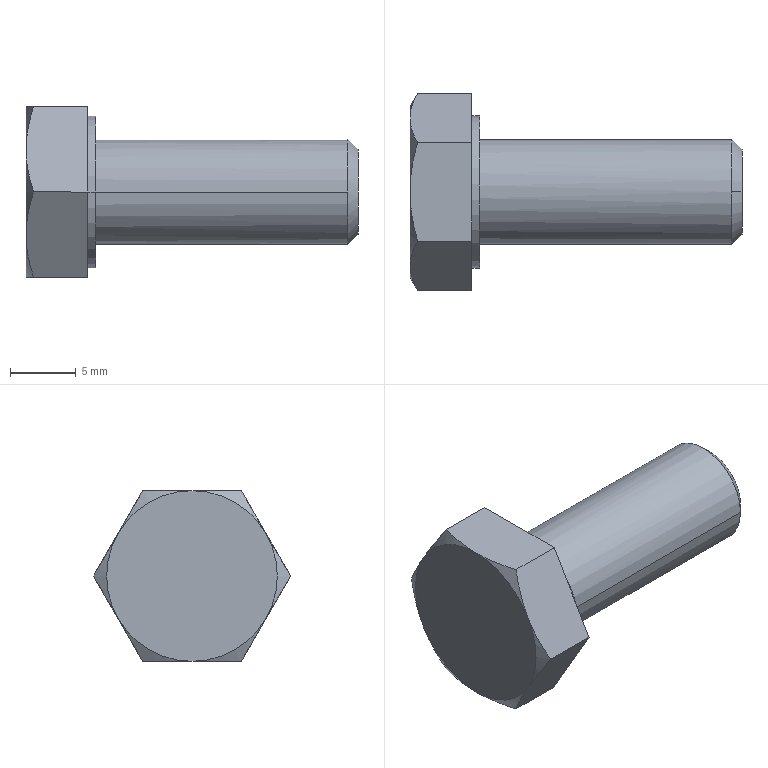Part | SolidWorks | features BaseBody 1 | 1 solid | 22 faces | box 25.3 x 15.011 x 13 mm | volume 1747 mm3 | plane 10 | cone 8 | cylinder 4 | commonest cylinder face diameters 8 x2 11.6 x2
STEP:
#1=CARTESIAN_POINT('',(0.,4.,0.));
#2=VERTEX_POINT('',#1);
#3=CARTESIAN_POINT('',(0.,-4.,0.));
#4=VERTEX_POINT('',#3);
#5=CARTESIAN_POINT('',(0.,0.,0.));
#6=DIRECTION('',(1.,0.,0.));
#7=DIRECTION('',(0.,1.,0.));
#8=AXIS2_PLACEMENT_3D('',#5,#6,#7);
#9=CIRCLE('',#8,4.);
#10=EDGE_CURVE('',#2,#4,#9,.T.);
#11=ORIENTED_EDGE('',*,*,#10,.T.);
#12=CARTESIAN_POINT('',(19.233,-4.,0.));
#13=VERTEX_POINT('',#12);
#14=CARTESIAN_POINT('',(10.625,-4.,0.));
#15=DIRECTION('',(1.,0.,0.));
#16=VECTOR('',#15,1000.);
#17=LINE('',#14,#16);
#18=EDGE_CURVE('',#4,#13,#17,.T.);
#19=ORIENTED_EDGE('',*,*,#18,.T.);
#20=CARTESIAN_POINT('',(19.233,0.,4.));
#21=VERTEX_POINT('',#20);
#22=CARTESIAN_POINT('',(19.233,0.,0.));
#23=DIRECTION('',(-1.,0.,0.));
#24=DIRECTION('',(0.,1.,0.));
#25=AXIS2_PLACEMENT_3D('',#22,#23,#24);
#26=CIRCLE('',#25,4.);
#27=EDGE_CURVE('',#13,#21,#26,.T.);
#28=ORIENTED_EDGE('',*,*,#27,.T.);
#29=CARTESIAN_POINT('',(19.233,4.,0.));
#30=VERTEX_POINT('',#29);
#31=CARTESIAN_POINT('',(19.233,0.,0.));
#32=DIRECTION('',(-1.,0.,0.));
#33=DIRECTION('',(0.,1.,0.));
#34=AXIS2_PLACEMENT_3D('',#31,#32,#33);
#35=CIRCLE('',#34,4.);
#36=EDGE_CURVE('',#21,#30,#35,.T.);
#37=ORIENTED_EDGE('',*,*,#36,.T.);
#38=CARTESIAN_POINT('',(10.625,4.,0.));
#39=DIRECTION('',(1.,0.,0.));
#40=VECTOR('',#39,1000.);
#41=LINE('',#38,#40);
#42=EDGE_CURVE('',#2,#30,#41,.T.);
#43=ORIENTED_EDGE('',*,*,#42,.F.);
#44=EDGE_LOOP('',(#11,#19,#28,#37,#43));
#45=FACE_OUTER_BOUND('',#44,.T.);
#46=CARTESIAN_POINT('',(10.625,0.,0.));
#47=DIRECTION('',(1.,0.,0.));
#48=DIRECTION('',(0.,1.,0.));
#49=AXIS2_PLACEMENT_3D('',#46,#47,#48);
#50=CYLINDRICAL_SURFACE('',#49,4.);
#51=ADVANCED_FACE('',(#45),#50,.T.);
#52=CARTESIAN_POINT('',(20.,0.,3.233));
#53=VERTEX_POINT('',#52);
#54=CARTESIAN_POINT('',(20.,0.,-3.233));
#55=VERTEX_POINT('',#54);
#56=CARTESIAN_POINT('',(20.,0.,0.));
#57=DIRECTION('',(-1.,0.,0.));
#58=DIRECTION('',(0.,0.,1.));
#59=AXIS2_PLACEMENT_3D('',#56,#57,#58);
#60=CIRCLE('',#59,3.233);
#61=EDGE_CURVE('',#53,#55,#60,.T.);
#62=ORIENTED_EDGE('',*,*,#61,.T.);
#63=CARTESIAN_POINT('',(19.233,0.,-4.));
#64=VERTEX_POINT('',#63);
#65=CARTESIAN_POINT('',(19.233,0.,-4.));
#66=DIRECTION('',(-0.7072,0.,-0.7071));
#67=VECTOR('',#66,1000.);
#68=LINE('',#65,#67);
#69=EDGE_CURVE('',#55,#64,#68,.T.);
#70=ORIENTED_EDGE('',*,*,#69,.T.);
#71=CARTESIAN_POINT('',(19.233,0.,0.));
#72=DIRECTION('',(-1.,0.,0.));
#73=DIRECTION('',(0.,1.,0.));
#74=AXIS2_PLACEMENT_3D('',#71,#72,#73);
#75=CIRCLE('',#74,4.);
#76=EDGE_CURVE('',#30,#64,#75,.T.);
#77=ORIENTED_EDGE('',*,*,#76,.F.);
#78=ORIENTED_EDGE('',*,*,#36,.F.);
#79=CARTESIAN_POINT('',(19.233,0.,4.));
#80=DIRECTION('',(-0.7072,0.,0.7071));
#81=VECTOR('',#80,1000.);
#82=LINE('',#79,#81);
#83=EDGE_CURVE('',#53,#21,#82,.T.);
#84=ORIENTED_EDGE('',*,*,#83,.F.);
#85=EDGE_LOOP('',(#62,#70,#77,#78,#84));
#86=FACE_OUTER_BOUND('',#85,.T.);
#87=CARTESIAN_POINT('',(19.233,0.,0.));
#88=DIRECTION('',(-1.,0.,0.));
#89=DIRECTION('',(0.,0.,1.));
#90=AXIS2_PLACEMENT_3D('',#87,#88,#89);
#91=CONICAL_SURFACE('',#90,4.,0.7853);
#92=ADVANCED_FACE('',(#86),#91,.T.);
#93=CARTESIAN_POINT('',(-0.6001,5.8,0.));
#94=VERTEX_POINT('',#93);
#95=CARTESIAN_POINT('',(-0.6001,-5.8,0.));
#96=VERTEX_POINT('',#95);
#97=CARTESIAN_POINT('',(-0.6001,0.,0.));
#98=DIRECTION('',(1.,0.,0.));
#99=DIRECTION('',(0.,1.,0.));
#100=AXIS2_PLACEMENT_3D('',#97,#98,#99);
#101=CIRCLE('',#100,5.8);
#102=EDGE_CURVE('',#94,#96,#101,.T.);
#103=ORIENTED_EDGE('',*,*,#102,.T.);
#104=CARTESIAN_POINT('',(0.,-5.8,0.));
#105=VERTEX_POINT('',#104);
#106=CARTESIAN_POINT('',(-0.3,-5.8,0.));
#107=DIRECTION('',(1.,0.,0.));
#108=VECTOR('',#107,1000.);
#109=LINE('',#106,#108);
#110=EDGE_CURVE('',#96,#105,#109,.T.);
#111=ORIENTED_EDGE('',*,*,#110,.T.);
#112=CARTESIAN_POINT('',(0.,5.8,0.));
#113=VERTEX_POINT('',#112);
#114=CARTESIAN_POINT('',(0.,0.,0.));
#115=DIRECTION('',(1.,0.,0.));
#116=DIRECTION('',(0.,1.,0.));
#117=AXIS2_PLACEMENT_3D('',#114,#115,#116);
#118=CIRCLE('',#117,5.8);
#119=EDGE_CURVE('',#113,#105,#118,.T.);
#120=ORIENTED_EDGE('',*,*,#119,.F.);
#121=CARTESIAN_POINT('',(-0.3,5.8,0.));
#122=DIRECTION('',(1.,0.,0.));
#123=VECTOR('',#122,1000.);
#124=LINE('',#121,#123);
#125=EDGE_CURVE('',#94,#113,#124,.T.);
#126=ORIENTED_EDGE('',*,*,#125,.F.);
#127=EDGE_LOOP('',(#103,#111,#120,#126));
#128=FACE_OUTER_BOUND('',#127,.T.);
#129=CARTESIAN_POINT('',(-0.3,0.,0.));
#130=DIRECTION('',(1.,0.,0.));
#131=DIRECTION('',(0.,1.,0.));
#132=AXIS2_PLACEMENT_3D('',#129,#130,#131);
#133=CYLINDRICAL_SURFACE('',#132,5.8);
#134=ADVANCED_FACE('',(#128),#133,.T.);
#135=ORIENTED_EDGE('',*,*,#18,.F.);
#136=CARTESIAN_POINT('',(0.,0.,0.));
#137=DIRECTION('',(1.,0.,0.));
#138=DIRECTION('',(0.,1.,0.));
#139=AXIS2_PLACEMENT_3D('',#136,#137,#138);
#140=CIRCLE('',#139,4.);
#141=EDGE_CURVE('',#4,#2,#140,.T.);
#142=ORIENTED_EDGE('',*,*,#141,.T.);
#143=ORIENTED_EDGE('',*,*,#42,.T.);
#144=ORIENTED_EDGE('',*,*,#76,.T.);
#145=CARTESIAN_POINT('',(19.233,0.,0.));
#146=DIRECTION('',(-1.,0.,0.));
#147=DIRECTION('',(0.,1.,0.));
#148=AXIS2_PLACEMENT_3D('',#145,#146,#147);
#149=CIRCLE('',#148,4.);
#150=EDGE_CURVE('',#64,#13,#149,.T.);
#151=ORIENTED_EDGE('',*,*,#150,.T.);
#152=EDGE_LOOP('',(#135,#142,#143,#144,#151));
#153=FACE_OUTER_BOUND('',#152,.T.);
#154=CARTESIAN_POINT('',(10.625,0.,0.));
#155=DIRECTION('',(1.,0.,0.));
#156=DIRECTION('',(0.,1.,0.));
#157=AXIS2_PLACEMENT_3D('',#154,#155,#156);
#158=CYLINDRICAL_SURFACE('',#157,4.);
#159=ADVANCED_FACE('',(#153),#158,.T.);
#160=ORIENTED_EDGE('',*,*,#69,.F.);
#161=CARTESIAN_POINT('',(20.,0.,0.));
#162=DIRECTION('',(-1.,0.,0.));
#163=DIRECTION('',(0.,0.,1.));
#164=AXIS2_PLACEMENT_3D('',#161,#162,#163);
#165=CIRCLE('',#164,3.233);
#166=EDGE_CURVE('',#55,#53,#165,.T.);
#167=ORIENTED_EDGE('',*,*,#166,.T.);
#168=ORIENTED_EDGE('',*,*,#83,.T.);
#169=ORIENTED_EDGE('',*,*,#27,.F.);
#170=ORIENTED_EDGE('',*,*,#150,.F.);
#171=EDGE_LOOP('',(#160,#167,#168,#169,#170));
#172=FACE_OUTER_BOUND('',#171,.T.);
#173=CARTESIAN_POINT('',(19.233,0.,0.));
#174=DIRECTION('',(-1.,0.,0.));
#175=DIRECTION('',(0.,0.,1.));
#176=AXIS2_PLACEMENT_3D('',#173,#174,#175);
#177=CONICAL_SURFACE('',#176,4.,0.7853);
#178=ADVANCED_FACE('',(#172),#177,.T.);
#179=ORIENTED_EDGE('',*,*,#10,.F.);
#180=ORIENTED_EDGE('',*,*,#141,.F.);
#181=EDGE_LOOP('',(#179,#180));
#182=FACE_BOUND('',#181,.T.);
#183=ORIENTED_EDGE('',*,*,#119,.T.);
#184=CARTESIAN_POINT('',(0.,0.,0.));
#185=DIRECTION('',(1.,0.,0.));
#186=DIRECTION('',(0.,1.,0.));
#187=AXIS2_PLACEMENT_3D('',#184,#185,#186);
#188=CIRCLE('',#187,5.8);
#189=EDGE_CURVE('',#105,#113,#188,.T.);
#190=ORIENTED_EDGE('',*,*,#189,.T.);
#191=EDGE_LOOP('',(#183,#190));
#192=FACE_OUTER_BOUND('',#191,.T.);
#193=CARTESIAN_POINT('',(0.,4.9,0.));
#194=DIRECTION('',(1.,0.,0.));
#195=DIRECTION('',(0.,1.,0.));
#196=AXIS2_PLACEMENT_3D('',#193,#194,#195);
#197=PLANE('',#196);
#198=ADVANCED_FACE('',(#182,#192),#197,.T.);
#199=ORIENTED_EDGE('',*,*,#61,.F.);
#200=ORIENTED_EDGE('',*,*,#166,.F.);
#201=EDGE_LOOP('',(#199,#200));
#202=FACE_OUTER_BOUND('',#201,.T.);
#203=CARTESIAN_POINT('',(20.,2.,0.));
#204=DIRECTION('',(1.,0.,0.));
#205=DIRECTION('',(0.,1.,0.));
#206=AXIS2_PLACEMENT_3D('',#203,#204,#205);
#207=PLANE('',#206);
#208=ADVANCED_FACE('',(#202),#207,.T.);
#209=ORIENTED_EDGE('',*,*,#110,.F.);
#210=CARTESIAN_POINT('',(-0.6001,0.,0.));
#211=DIRECTION('',(1.,0.,0.));
#212=DIRECTION('',(0.,1.,0.));
#213=AXIS2_PLACEMENT_3D('',#210,#211,#212);
#214=CIRCLE('',#213,5.8);
#215=EDGE_CURVE('',#96,#94,#214,.T.);
#216=ORIENTED_EDGE('',*,*,#215,.T.);
#217=ORIENTED_EDGE('',*,*,#125,.T.);
#218=ORIENTED_EDGE('',*,*,#189,.F.);
#219=EDGE_LOOP('',(#209,#216,#217,#218));
#220=FACE_OUTER_BOUND('',#219,.T.);
#221=CARTESIAN_POINT('',(-0.3,0.,0.));
#222=DIRECTION('',(1.,0.,0.));
#223=DIRECTION('',(0.,1.,0.));
#224=AXIS2_PLACEMENT_3D('',#221,#222,#223);
#225=CYLINDRICAL_SURFACE('',#224,5.8);
#226=ADVANCED_FACE('',(#220),#225,.T.);
#227=ORIENTED_EDGE('',*,*,#102,.F.);
#228=ORIENTED_EDGE('',*,*,#215,.F.);
#229=EDGE_LOOP('',(#227,#228));
#230=FACE_BOUND('',#229,.T.);
#231=CARTESIAN_POINT('',(-0.6001,-3.753,-6.5));
#232=VERTEX_POINT('',#231);
#233=CARTESIAN_POINT('',(-0.6001,3.753,-6.5));
#234=VERTEX_POINT('',#233);
#235=CARTESIAN_POINT('',(-0.6001,0.,-6.5));
#236=DIRECTION('',(0.,1.,0.));
#237=VECTOR('',#236,1000.);
#238=LINE('',#235,#237);
#239=EDGE_CURVE('',#232,#234,#238,.T.);
#240=ORIENTED_EDGE('',*,*,#239,.T.);
#241=CARTESIAN_POINT('',(-0.6001,7.506,0.));
#242=VERTEX_POINT('',#241);
#243=CARTESIAN_POINT('',(-0.6001,3.753,-6.5));
#244=DIRECTION('',(0.,0.5,0.866));
#245=VECTOR('',#244,1000.);
#246=LINE('',#243,#245);
#247=EDGE_CURVE('',#234,#242,#246,.T.);
#248=ORIENTED_EDGE('',*,*,#247,.T.);
#249=CARTESIAN_POINT('',(-0.6001,3.753,6.5));
#250=VERTEX_POINT('',#249);
#251=CARTESIAN_POINT('',(-0.6001,7.506,0.));
#252=DIRECTION('',(0.,-0.5,0.866));
#253=VECTOR('',#252,1000.);
#254=LINE('',#251,#253);
#255=EDGE_CURVE('',#242,#250,#254,.T.);
#256=ORIENTED_EDGE('',*,*,#255,.T.);
#257=CARTESIAN_POINT('',(-0.6001,-3.753,6.5));
#258=VERTEX_POINT('',#257);
#259=CARTESIAN_POINT('',(-0.6001,0.,6.5));
#260=DIRECTION('',(0.,-1.,0.));
#261=VECTOR('',#260,1000.);
#262=LINE('',#259,#261);
#263=EDGE_CURVE('',#250,#258,#262,.T.);
#264=ORIENTED_EDGE('',*,*,#263,.T.);
#265=CARTESIAN_POINT('',(-0.6001,-7.506,0.));
#266=VERTEX_POINT('',#265);
#267=CARTESIAN_POINT('',(-0.6001,-3.753,6.5));
#268=DIRECTION('',(0.,-0.5,-0.866));
#269=VECTOR('',#268,1000.);
#270=LINE('',#267,#269);
#271=EDGE_CURVE('',#258,#266,#270,.T.);
#272=ORIENTED_EDGE('',*,*,#271,.T.);
#273=CARTESIAN_POINT('',(-0.6001,-7.506,0.));
#274=DIRECTION('',(0.,0.5,-0.866));
#275=VECTOR('',#274,1000.);
#276=LINE('',#273,#275);
#277=EDGE_CURVE('',#266,#232,#276,.T.);
#278=ORIENTED_EDGE('',*,*,#277,.T.);
#279=EDGE_LOOP('',(#240,#248,#256,#264,#272,#278));
#280=FACE_OUTER_BOUND('',#279,.T.);
#281=CARTESIAN_POINT('',(-0.6001,0.,0.));
#282=DIRECTION('',(1.,0.,0.));
#283=DIRECTION('',(0.,1.,0.));
#284=AXIS2_PLACEMENT_3D('',#281,#282,#283);
#285=PLANE('',#284);
#286=ADVANCED_FACE('',(#230,#280),#285,.T.);
#287=ORIENTED_EDGE('',*,*,#247,.F.);
#288=CARTESIAN_POINT('',(-4.72,3.753,-6.5));
#289=VERTEX_POINT('',#288);
#290=CARTESIAN_POINT('',(-0.6001,3.753,-6.5));
#291=DIRECTION('',(-1.,0.,0.));
#292=VECTOR('',#291,1000.);
#293=LINE('',#290,#292);
#294=EDGE_CURVE('',#234,#289,#293,.T.);
#295=ORIENTED_EDGE('',*,*,#294,.T.);
#296=CARTESIAN_POINT('',(-5.3,5.629,-3.25));
#297=VERTEX_POINT('',#296);
#298=CARTESIAN_POINT('',(-4.72,3.753,-6.5));
#299=CARTESIAN_POINT('',(-5.073,4.366,-5.438));
#300=CARTESIAN_POINT('',(-5.3,4.989,-4.359));
#301=CARTESIAN_POINT('',(-5.3,5.629,-3.25));
#302=B_SPLINE_CURVE_WITH_KNOTS('',3,(#298,#299,#300,#301),.UNSPECIFIED.,.F.,.F.,(4,4),(0.,0.003797),.UNSPECIFIED.);
#303=EDGE_CURVE('',#289,#297,#302,.T.);
#304=ORIENTED_EDGE('',*,*,#303,.T.);
#305=CARTESIAN_POINT('',(-4.72,7.506,0.));
#306=VERTEX_POINT('',#305);
#307=CARTESIAN_POINT('',(-5.3,5.629,-3.25));
#308=CARTESIAN_POINT('',(-5.3,6.27,-2.141));
#309=CARTESIAN_POINT('',(-5.073,6.892,-1.062));
#310=CARTESIAN_POINT('',(-4.72,7.506,0.));
#311=B_SPLINE_CURVE_WITH_KNOTS('',3,(#307,#308,#309,#310),.UNSPECIFIED.,.F.,.F.,(4,4),(0.,0.003797),.UNSPECIFIED.);
#312=EDGE_CURVE('',#297,#306,#311,.T.);
#313=ORIENTED_EDGE('',*,*,#312,.T.);
#314=CARTESIAN_POINT('',(-0.6001,7.506,0.));
#315=DIRECTION('',(1.,0.,0.));
#316=VECTOR('',#315,1000.);
#317=LINE('',#314,#316);
#318=EDGE_CURVE('',#306,#242,#317,.T.);
#319=ORIENTED_EDGE('',*,*,#318,.T.);
#320=EDGE_LOOP('',(#287,#295,#304,#313,#319));
#321=FACE_OUTER_BOUND('',#320,.T.);
#322=CARTESIAN_POINT('',(-0.6001,3.753,-6.5));
#323=DIRECTION('',(0.,0.866,-0.5));
#324=DIRECTION('',(0.,0.5,0.866));
#325=AXIS2_PLACEMENT_3D('',#322,#323,#324);
#326=PLANE('',#325);
#327=ADVANCED_FACE('',(#321),#326,.T.);
#328=ORIENTED_EDGE('',*,*,#239,.F.);
#329=CARTESIAN_POINT('',(-4.72,-3.753,-6.5));
#330=VERTEX_POINT('',#329);
#331=CARTESIAN_POINT('',(-0.6001,-3.753,-6.5));
#332=DIRECTION('',(-1.,0.,0.));
#333=VECTOR('',#332,1000.);
#334=LINE('',#331,#333);
#335=EDGE_CURVE('',#232,#330,#334,.T.);
#336=ORIENTED_EDGE('',*,*,#335,.T.);
#337=CARTESIAN_POINT('',(-5.3,0.,-6.5));
#338=VERTEX_POINT('',#337);
#339=CARTESIAN_POINT('',(-4.72,-3.753,-6.5));
#340=CARTESIAN_POINT('',(-5.073,-2.527,-6.5));
#341=CARTESIAN_POINT('',(-5.3,-1.281,-6.5));
#342=CARTESIAN_POINT('',(-5.3,0.,-6.5));
#343=B_SPLINE_CURVE_WITH_KNOTS('',3,(#339,#340,#341,#342),.UNSPECIFIED.,.F.,.F.,(4,4),(0.,0.003797),.UNSPECIFIED.);
#344=EDGE_CURVE('',#330,#338,#343,.T.);
#345=ORIENTED_EDGE('',*,*,#344,.T.);
#346=CARTESIAN_POINT('',(-5.3,0.,-6.5));
#347=CARTESIAN_POINT('',(-5.3,1.281,-6.5));
#348=CARTESIAN_POINT('',(-5.073,2.527,-6.5));
#349=CARTESIAN_POINT('',(-4.72,3.753,-6.5));
#350=B_SPLINE_CURVE_WITH_KNOTS('',3,(#346,#347,#348,#349),.UNSPECIFIED.,.F.,.F.,(4,4),(0.,0.003797),.UNSPECIFIED.);
#351=EDGE_CURVE('',#338,#289,#350,.T.);
#352=ORIENTED_EDGE('',*,*,#351,.T.);
#353=ORIENTED_EDGE('',*,*,#294,.F.);
#354=EDGE_LOOP('',(#328,#336,#345,#352,#353));
#355=FACE_OUTER_BOUND('',#354,.T.);
#356=CARTESIAN_POINT('',(-0.6001,-3.753,-6.5));
#357=DIRECTION('',(0.,0.,-1.));
#358=DIRECTION('',(0.,1.,0.));
#359=AXIS2_PLACEMENT_3D('',#356,#357,#358);
#360=PLANE('',#359);
#361=ADVANCED_FACE('',(#355),#360,.T.);
#362=CARTESIAN_POINT('',(-4.72,-7.506,0.));
#363=VERTEX_POINT('',#362);
#364=CARTESIAN_POINT('',(-0.6001,-7.506,0.));
#365=DIRECTION('',(-1.,0.,0.));
#366=VECTOR('',#365,1000.);
#367=LINE('',#364,#366);
#368=EDGE_CURVE('',#266,#363,#367,.T.);
#369=ORIENTED_EDGE('',*,*,#368,.T.);
#370=CARTESIAN_POINT('',(-5.3,-5.629,-3.25));
#371=VERTEX_POINT('',#370);
#372=CARTESIAN_POINT('',(-4.72,-7.506,0.));
#373=CARTESIAN_POINT('',(-5.073,-6.892,-1.062));
#374=CARTESIAN_POINT('',(-5.3,-6.27,-2.141));
#375=CARTESIAN_POINT('',(-5.3,-5.629,-3.25));
#376=B_SPLINE_CURVE_WITH_KNOTS('',3,(#372,#373,#374,#375),.UNSPECIFIED.,.F.,.F.,(4,4),(0.,0.003797),.UNSPECIFIED.);
#377=EDGE_CURVE('',#363,#371,#376,.T.);
#378=ORIENTED_EDGE('',*,*,#377,.T.);
#379=CARTESIAN_POINT('',(-5.3,-5.629,-3.25));
#380=CARTESIAN_POINT('',(-5.3,-4.989,-4.359));
#381=CARTESIAN_POINT('',(-5.073,-4.366,-5.438));
#382=CARTESIAN_POINT('',(-4.72,-3.753,-6.5));
#383=B_SPLINE_CURVE_WITH_KNOTS('',3,(#379,#380,#381,#382),.UNSPECIFIED.,.F.,.F.,(4,4),(0.,0.003797),.UNSPECIFIED.);
#384=EDGE_CURVE('',#371,#330,#383,.T.);
#385=ORIENTED_EDGE('',*,*,#384,.T.);
#386=ORIENTED_EDGE('',*,*,#335,.F.);
#387=ORIENTED_EDGE('',*,*,#277,.F.);
#388=EDGE_LOOP('',(#369,#378,#385,#386,#387));
#389=FACE_OUTER_BOUND('',#388,.T.);
#390=CARTESIAN_POINT('',(-0.6001,-7.506,0.));
#391=DIRECTION('',(0.,-0.866,-0.5));
#392=DIRECTION('',(0.,0.5,-0.866));
#393=AXIS2_PLACEMENT_3D('',#390,#391,#392);
#394=PLANE('',#393);
#395=ADVANCED_FACE('',(#389),#394,.T.);
#396=CARTESIAN_POINT('',(-4.72,-3.753,6.5));
#397=VERTEX_POINT('',#396);
#398=CARTESIAN_POINT('',(-0.6001,-3.753,6.5));
#399=DIRECTION('',(-1.,0.,0.));
#400=VECTOR('',#399,1000.);
#401=LINE('',#398,#400);
#402=EDGE_CURVE('',#258,#397,#401,.T.);
#403=ORIENTED_EDGE('',*,*,#402,.T.);
#404=CARTESIAN_POINT('',(-5.3,-5.629,3.25));
#405=VERTEX_POINT('',#404);
#406=CARTESIAN_POINT('',(-4.72,-3.753,6.5));
#407=CARTESIAN_POINT('',(-5.073,-4.366,5.438));
#408=CARTESIAN_POINT('',(-5.3,-4.989,4.359));
#409=CARTESIAN_POINT('',(-5.3,-5.629,3.25));
#410=B_SPLINE_CURVE_WITH_KNOTS('',3,(#406,#407,#408,#409),.UNSPECIFIED.,.F.,.F.,(4,4),(0.,0.003797),.UNSPECIFIED.);
#411=EDGE_CURVE('',#397,#405,#410,.T.);
#412=ORIENTED_EDGE('',*,*,#411,.T.);
#413=CARTESIAN_POINT('',(-5.3,-5.629,3.25));
#414=CARTESIAN_POINT('',(-5.3,-6.27,2.141));
#415=CARTESIAN_POINT('',(-5.073,-6.892,1.062));
#416=CARTESIAN_POINT('',(-4.72,-7.506,0.));
#417=B_SPLINE_CURVE_WITH_KNOTS('',3,(#413,#414,#415,#416),.UNSPECIFIED.,.F.,.F.,(4,4),(0.,0.003797),.UNSPECIFIED.);
#418=EDGE_CURVE('',#405,#363,#417,.T.);
#419=ORIENTED_EDGE('',*,*,#418,.T.);
#420=ORIENTED_EDGE('',*,*,#368,.F.);
#421=ORIENTED_EDGE('',*,*,#271,.F.);
#422=EDGE_LOOP('',(#403,#412,#419,#420,#421));
#423=FACE_OUTER_BOUND('',#422,.T.);
#424=CARTESIAN_POINT('',(-0.6001,-3.753,6.5));
#425=DIRECTION('',(0.,-0.866,0.5));
#426=DIRECTION('',(0.,-0.5,-0.866));
#427=AXIS2_PLACEMENT_3D('',#424,#425,#426);
#428=PLANE('',#427);
#429=ADVANCED_FACE('',(#423),#428,.T.);
#430=CARTESIAN_POINT('',(-4.72,3.753,6.5));
#431=VERTEX_POINT('',#430);
#432=CARTESIAN_POINT('',(-0.6001,3.753,6.5));
#433=DIRECTION('',(-1.,0.,0.));
#434=VECTOR('',#433,1000.);
#435=LINE('',#432,#434);
#436=EDGE_CURVE('',#250,#431,#435,.T.);
#437=ORIENTED_EDGE('',*,*,#436,.T.);
#438=CARTESIAN_POINT('',(-5.3,0.,6.5));
#439=VERTEX_POINT('',#438);
#440=CARTESIAN_POINT('',(-4.72,3.753,6.5));
#441=CARTESIAN_POINT('',(-5.073,2.527,6.5));
#442=CARTESIAN_POINT('',(-5.3,1.281,6.5));
#443=CARTESIAN_POINT('',(-5.3,0.,6.5));
#444=B_SPLINE_CURVE_WITH_KNOTS('',3,(#440,#441,#442,#443),.UNSPECIFIED.,.F.,.F.,(4,4),(0.,0.003797),.UNSPECIFIED.);
#445=EDGE_CURVE('',#431,#439,#444,.T.);
#446=ORIENTED_EDGE('',*,*,#445,.T.);
#447=CARTESIAN_POINT('',(-5.3,0.,6.5));
#448=CARTESIAN_POINT('',(-5.3,-1.281,6.5));
#449=CARTESIAN_POINT('',(-5.073,-2.527,6.5));
#450=CARTESIAN_POINT('',(-4.72,-3.753,6.5));
#451=B_SPLINE_CURVE_WITH_KNOTS('',3,(#447,#448,#449,#450),.UNSPECIFIED.,.F.,.F.,(4,4),(0.,0.003797),.UNSPECIFIED.);
#452=EDGE_CURVE('',#439,#397,#451,.T.);
#453=ORIENTED_EDGE('',*,*,#452,.T.);
#454=ORIENTED_EDGE('',*,*,#402,.F.);
#455=ORIENTED_EDGE('',*,*,#263,.F.);
#456=EDGE_LOOP('',(#437,#446,#453,#454,#455));
#457=FACE_OUTER_BOUND('',#456,.T.);
#458=CARTESIAN_POINT('',(-0.6001,3.753,6.5));
#459=DIRECTION('',(0.,0.,1.));
#460=DIRECTION('',(0.,-1.,0.));
#461=AXIS2_PLACEMENT_3D('',#458,#459,#460);
#462=PLANE('',#461);
#463=ADVANCED_FACE('',(#457),#462,.T.);
#464=ORIENTED_EDGE('',*,*,#255,.F.);
#465=ORIENTED_EDGE('',*,*,#318,.F.);
#466=CARTESIAN_POINT('',(-5.3,5.629,3.25));
#467=VERTEX_POINT('',#466);
#468=CARTESIAN_POINT('',(-4.72,7.506,0.));
#469=CARTESIAN_POINT('',(-5.073,6.892,1.062));
#470=CARTESIAN_POINT('',(-5.3,6.27,2.141));
#471=CARTESIAN_POINT('',(-5.3,5.629,3.25));
#472=B_SPLINE_CURVE_WITH_KNOTS('',3,(#468,#469,#470,#471),.UNSPECIFIED.,.F.,.F.,(4,4),(0.,0.003797),.UNSPECIFIED.);
#473=EDGE_CURVE('',#306,#467,#472,.T.);
#474=ORIENTED_EDGE('',*,*,#473,.T.);
#475=CARTESIAN_POINT('',(-5.3,5.629,3.25));
#476=CARTESIAN_POINT('',(-5.3,4.989,4.359));
#477=CARTESIAN_POINT('',(-5.073,4.366,5.438));
#478=CARTESIAN_POINT('',(-4.72,3.753,6.5));
#479=B_SPLINE_CURVE_WITH_KNOTS('',3,(#475,#476,#477,#478),.UNSPECIFIED.,.F.,.F.,(4,4),(0.,0.003797),.UNSPECIFIED.);
#480=EDGE_CURVE('',#467,#431,#479,.T.);
#481=ORIENTED_EDGE('',*,*,#480,.T.);
#482=ORIENTED_EDGE('',*,*,#436,.F.);
#483=EDGE_LOOP('',(#464,#465,#474,#481,#482));
#484=FACE_OUTER_BOUND('',#483,.T.);
#485=CARTESIAN_POINT('',(-0.6001,7.506,0.));
#486=DIRECTION('',(0.,0.866,0.5));
#487=DIRECTION('',(0.,-0.5,0.866));
#488=AXIS2_PLACEMENT_3D('',#485,#486,#487);
#489=PLANE('',#488);
#490=ADVANCED_FACE('',(#484),#489,.T.);
#491=CARTESIAN_POINT('',(-5.3,0.,0.));
#492=DIRECTION('',(1.,0.,0.));
#493=DIRECTION('',(0.,0.,-1.));
#494=AXIS2_PLACEMENT_3D('',#491,#492,#493);
#495=CIRCLE('',#494,6.5);
#496=EDGE_CURVE('',#297,#467,#495,.T.);
#497=ORIENTED_EDGE('',*,*,#496,.T.);
#498=ORIENTED_EDGE('',*,*,#473,.F.);
#499=ORIENTED_EDGE('',*,*,#312,.F.);
#500=EDGE_LOOP('',(#497,#498,#499));
#501=FACE_OUTER_BOUND('',#500,.T.);
#502=CARTESIAN_POINT('',(-4.716,0.,0.));
#503=DIRECTION('',(1.,0.,0.));
#504=DIRECTION('',(0.,0.,-1.));
#505=AXIS2_PLACEMENT_3D('',#502,#503,#504);
#506=CONICAL_SURFACE('',#505,7.512,1.047);
#507=ADVANCED_FACE('',(#501),#506,.T.);
#508=CARTESIAN_POINT('',(-5.3,0.,0.));
#509=DIRECTION('',(1.,0.,0.));
#510=DIRECTION('',(0.,0.,-1.));
#511=AXIS2_PLACEMENT_3D('',#508,#509,#510);
#512=CIRCLE('',#511,6.5);
#513=EDGE_CURVE('',#338,#297,#512,.T.);
#514=ORIENTED_EDGE('',*,*,#513,.T.);
#515=ORIENTED_EDGE('',*,*,#303,.F.);
#516=ORIENTED_EDGE('',*,*,#351,.F.);
#517=EDGE_LOOP('',(#514,#515,#516));
#518=FACE_OUTER_BOUND('',#517,.T.);
#519=CARTESIAN_POINT('',(-4.716,0.,0.));
#520=DIRECTION('',(1.,0.,0.));
#521=DIRECTION('',(0.,0.,-1.));
#522=AXIS2_PLACEMENT_3D('',#519,#520,#521);
#523=CONICAL_SURFACE('',#522,7.512,1.047);
#524=ADVANCED_FACE('',(#518),#523,.T.);
#525=ORIENTED_EDGE('',*,*,#384,.F.);
#526=CARTESIAN_POINT('',(-5.3,0.,0.));
#527=DIRECTION('',(1.,0.,0.));
#528=DIRECTION('',(0.,0.,-1.));
#529=AXIS2_PLACEMENT_3D('',#526,#527,#528);
#530=CIRCLE('',#529,6.5);
#531=EDGE_CURVE('',#371,#338,#530,.T.);
#532=ORIENTED_EDGE('',*,*,#531,.T.);
#533=ORIENTED_EDGE('',*,*,#344,.F.);
#534=EDGE_LOOP('',(#525,#532,#533));
#535=FACE_OUTER_BOUND('',#534,.T.);
#536=CARTESIAN_POINT('',(-4.716,0.,0.));
#537=DIRECTION('',(1.,0.,0.));
#538=DIRECTION('',(0.,0.,-1.));
#539=AXIS2_PLACEMENT_3D('',#536,#537,#538);
#540=CONICAL_SURFACE('',#539,7.512,1.047);
#541=ADVANCED_FACE('',(#535),#540,.T.);
#542=ORIENTED_EDGE('',*,*,#418,.F.);
#543=CARTESIAN_POINT('',(-5.3,0.,0.));
#544=DIRECTION('',(1.,0.,0.));
#545=DIRECTION('',(0.,0.,-1.));
#546=AXIS2_PLACEMENT_3D('',#543,#544,#545);
#547=CIRCLE('',#546,6.5);
#548=EDGE_CURVE('',#405,#371,#547,.T.);
#549=ORIENTED_EDGE('',*,*,#548,.T.);
#550=ORIENTED_EDGE('',*,*,#377,.F.);
#551=EDGE_LOOP('',(#542,#549,#550));
#552=FACE_OUTER_BOUND('',#551,.T.);
#553=CARTESIAN_POINT('',(-4.716,0.,0.));
#554=DIRECTION('',(1.,0.,0.));
#555=DIRECTION('',(0.,0.,-1.));
#556=AXIS2_PLACEMENT_3D('',#553,#554,#555);
#557=CONICAL_SURFACE('',#556,7.512,1.047);
#558=ADVANCED_FACE('',(#552),#557,.T.);
#559=ORIENTED_EDGE('',*,*,#452,.F.);
#560=CARTESIAN_POINT('',(-5.3,0.,0.));
#561=DIRECTION('',(1.,0.,0.));
#562=DIRECTION('',(0.,0.,-1.));
#563=AXIS2_PLACEMENT_3D('',#560,#561,#562);
#564=CIRCLE('',#563,6.5);
#565=EDGE_CURVE('',#439,#405,#564,.T.);
#566=ORIENTED_EDGE('',*,*,#565,.T.);
#567=ORIENTED_EDGE('',*,*,#411,.F.);
#568=EDGE_LOOP('',(#559,#566,#567));
#569=FACE_OUTER_BOUND('',#568,.T.);
#570=CARTESIAN_POINT('',(-4.716,0.,0.));
#571=DIRECTION('',(1.,0.,0.));
#572=DIRECTION('',(0.,0.,-1.));
#573=AXIS2_PLACEMENT_3D('',#570,#571,#572);
#574=CONICAL_SURFACE('',#573,7.512,1.047);
#575=ADVANCED_FACE('',(#569),#574,.T.);
#576=CARTESIAN_POINT('',(-5.3,0.,0.));
#577=DIRECTION('',(1.,0.,0.));
#578=DIRECTION('',(0.,0.,-1.));
#579=AXIS2_PLACEMENT_3D('',#576,#577,#578);
#580=CIRCLE('',#579,6.5);
#581=EDGE_CURVE('',#467,#439,#580,.T.);
#582=ORIENTED_EDGE('',*,*,#581,.T.);
#583=ORIENTED_EDGE('',*,*,#445,.F.);
#584=ORIENTED_EDGE('',*,*,#480,.F.);
#585=EDGE_LOOP('',(#582,#583,#584));
#586=FACE_OUTER_BOUND('',#585,.T.);
#587=CARTESIAN_POINT('',(-4.716,0.,0.));
#588=DIRECTION('',(1.,0.,0.));
#589=DIRECTION('',(0.,0.,-1.));
#590=AXIS2_PLACEMENT_3D('',#587,#588,#589);
#591=CONICAL_SURFACE('',#590,7.512,1.047);
#592=ADVANCED_FACE('',(#586),#591,.T.);
#593=ORIENTED_EDGE('',*,*,#496,.F.);
#594=ORIENTED_EDGE('',*,*,#513,.F.);
#595=ORIENTED_EDGE('',*,*,#531,.F.);
#596=ORIENTED_EDGE('',*,*,#548,.F.);
#597=ORIENTED_EDGE('',*,*,#565,.F.);
#598=ORIENTED_EDGE('',*,*,#581,.F.);
#599=EDGE_LOOP('',(#593,#594,#595,#596,#597,#598));
#600=FACE_OUTER_BOUND('',#599,.T.);
#601=CARTESIAN_POINT('',(-5.3,0.,0.));
#602=DIRECTION('',(1.,0.,0.));
#603=DIRECTION('',(0.,1.,0.));
#604=AXIS2_PLACEMENT_3D('',#601,#602,#603);
#605=PLANE('',#604);
#606=ADVANCED_FACE('',(#600),#605,.F.);
#607=CLOSED_SHELL('',(#51,#92,#134,#159,#178,#198,#208,#226,#286,#327,#361,#395,#429,#463,#490,#507,#524,#541,#558,#575,#592,#606));
#608=MANIFOLD_SOLID_BREP('',#607);
#609=CARTESIAN_POINT('',(0.,0.,0.));
#610=DIRECTION('',(0.,0.,1.));
#611=DIRECTION('',(1.,0.,0.));
#612=AXIS2_PLACEMENT_3D('',#609,#610,#611);
#613=(LENGTH_UNIT()NAMED_UNIT(*)SI_UNIT(.MILLI.,.METRE.));
#614=UNCERTAINTY_MEASURE_WITH_UNIT(LENGTH_MEASURE(0.00001),#613,'','');
#615=(NAMED_UNIT(*)PLANE_ANGLE_UNIT()SI_UNIT($,.RADIAN.));
#616=(NAMED_UNIT(*)SI_UNIT($,.STERADIAN.)SOLID_ANGLE_UNIT());
#617=(GEOMETRIC_REPRESENTATION_CONTEXT(3)GLOBAL_UNCERTAINTY_ASSIGNED_CONTEXT((#614))GLOBAL_UNIT_ASSIGNED_CONTEXT((#613,#615,#616))REPRESENTATION_CONTEXT('',''));
#618=ADVANCED_BREP_SHAPE_REPRESENTATION('',(#608,#612),#617);